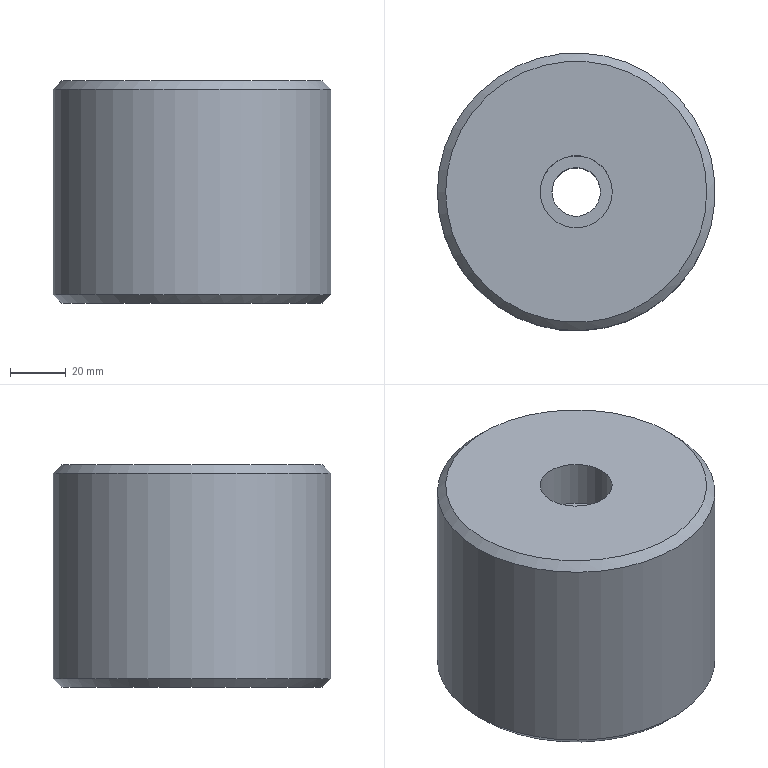Part | STEP file | solid 130 | 1 solid | 8 faces | box 100 x 100 x 80 mm | volume 601369 mm3 | plane 3 | cylinder 3 | cone 2 | commonest cylinder face diameters 17.5 x1 26 x1 100 x1